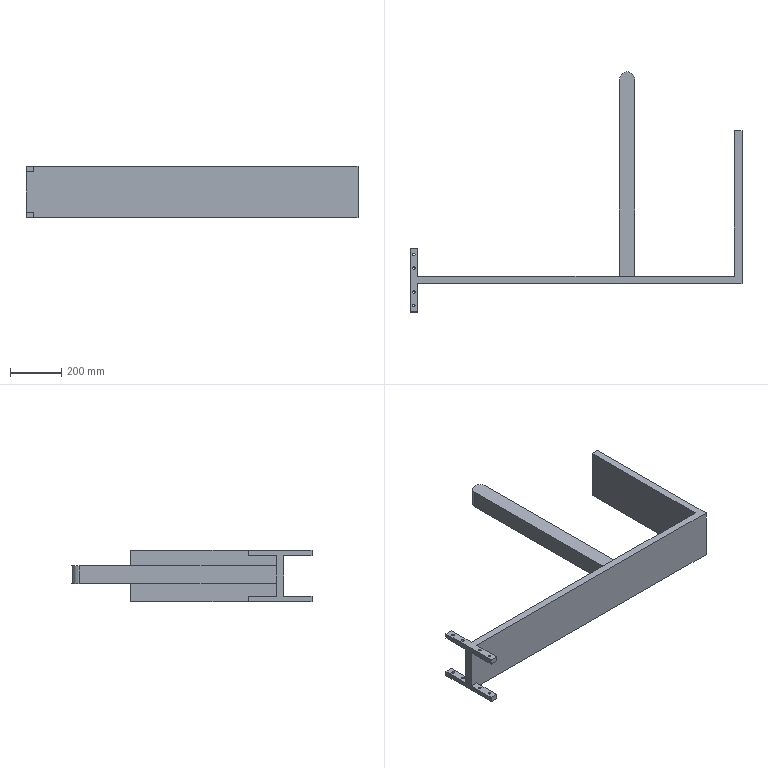Part | SolidWorks | features ICE 3, Extrusion 1 | 1 solid | 41 faces | box 1300 x 940 x 200 mm | volume 14804394 mm3 | plane 24 | cylinder 17 | commonest cylinder face diameters 10 x16 60 x1
STEP:
#1=CARTESIAN_POINT('',(-1438.05,-1320.198,-180.));
#2=VERTEX_POINT('',#1);
#3=CARTESIAN_POINT('',(-1428.05,-1320.198,-180.));
#4=VERTEX_POINT('',#3);
#5=CARTESIAN_POINT('',(-1433.05,-1320.198,-180.));
#6=DIRECTION('',(0.,0.,1.));
#7=DIRECTION('',(0.,-1.,0.));
#8=AXIS2_PLACEMENT_3D('',#5,#6,#7);
#9=CIRCLE('',#8,5.);
#10=EDGE_CURVE('',#2,#4,#9,.T.);
#11=ORIENTED_EDGE('',*,*,#10,.T.);
#12=CARTESIAN_POINT('',(-1428.05,-1320.198,-200.));
#13=VERTEX_POINT('',#12);
#14=CARTESIAN_POINT('',(-1428.05,-1320.198,30.));
#15=DIRECTION('',(0.,0.,-1.));
#16=VECTOR('',#15,1000.);
#17=LINE('',#14,#16);
#18=EDGE_CURVE('',#4,#13,#17,.T.);
#19=ORIENTED_EDGE('',*,*,#18,.T.);
#20=CARTESIAN_POINT('',(-1438.05,-1320.198,-200.));
#21=VERTEX_POINT('',#20);
#22=CARTESIAN_POINT('',(-1433.05,-1320.198,-200.));
#23=DIRECTION('',(0.,0.,-1.));
#24=DIRECTION('',(-1.,0.,0.));
#25=AXIS2_PLACEMENT_3D('',#22,#23,#24);
#26=CIRCLE('',#25,5.);
#27=EDGE_CURVE('',#13,#21,#26,.T.);
#28=ORIENTED_EDGE('',*,*,#27,.T.);
#29=CARTESIAN_POINT('',(-1438.05,-1320.198,30.));
#30=DIRECTION('',(0.,0.,-1.));
#31=VECTOR('',#30,1000.);
#32=LINE('',#29,#31);
#33=EDGE_CURVE('',#2,#21,#32,.T.);
#34=ORIENTED_EDGE('',*,*,#33,.F.);
#35=EDGE_LOOP('',(#11,#19,#28,#34));
#36=FACE_OUTER_BOUND('',#35,.T.);
#37=CARTESIAN_POINT('',(-1433.05,-1320.198,30.));
#38=DIRECTION('',(0.,0.,-1.));
#39=DIRECTION('',(-1.,0.,0.));
#40=AXIS2_PLACEMENT_3D('',#37,#38,#39);
#41=CYLINDRICAL_SURFACE('',#40,5.);
#42=ADVANCED_FACE('',(#36),#41,.F.);
#43=CARTESIAN_POINT('',(-1438.05,-1373.198,-180.));
#44=VERTEX_POINT('',#43);
#45=CARTESIAN_POINT('',(-1428.05,-1373.198,-180.));
#46=VERTEX_POINT('',#45);
#47=CARTESIAN_POINT('',(-1433.05,-1373.198,-180.));
#48=DIRECTION('',(0.,0.,1.));
#49=DIRECTION('',(0.,-1.,0.));
#50=AXIS2_PLACEMENT_3D('',#47,#48,#49);
#51=CIRCLE('',#50,5.);
#52=EDGE_CURVE('',#44,#46,#51,.T.);
#53=ORIENTED_EDGE('',*,*,#52,.T.);
#54=CARTESIAN_POINT('',(-1428.05,-1373.198,-200.));
#55=VERTEX_POINT('',#54);
#56=CARTESIAN_POINT('',(-1428.05,-1373.198,30.));
#57=DIRECTION('',(0.,0.,-1.));
#58=VECTOR('',#57,1000.);
#59=LINE('',#56,#58);
#60=EDGE_CURVE('',#46,#55,#59,.T.);
#61=ORIENTED_EDGE('',*,*,#60,.T.);
#62=CARTESIAN_POINT('',(-1438.05,-1373.198,-200.));
#63=VERTEX_POINT('',#62);
#64=CARTESIAN_POINT('',(-1433.05,-1373.198,-200.));
#65=DIRECTION('',(0.,0.,-1.));
#66=DIRECTION('',(-1.,0.,0.));
#67=AXIS2_PLACEMENT_3D('',#64,#65,#66);
#68=CIRCLE('',#67,5.);
#69=EDGE_CURVE('',#55,#63,#68,.T.);
#70=ORIENTED_EDGE('',*,*,#69,.T.);
#71=CARTESIAN_POINT('',(-1438.05,-1373.198,30.));
#72=DIRECTION('',(0.,0.,-1.));
#73=VECTOR('',#72,1000.);
#74=LINE('',#71,#73);
#75=EDGE_CURVE('',#44,#63,#74,.T.);
#76=ORIENTED_EDGE('',*,*,#75,.F.);
#77=EDGE_LOOP('',(#53,#61,#70,#76));
#78=FACE_OUTER_BOUND('',#77,.T.);
#79=CARTESIAN_POINT('',(-1433.05,-1373.198,30.));
#80=DIRECTION('',(0.,0.,-1.));
#81=DIRECTION('',(-1.,0.,0.));
#82=AXIS2_PLACEMENT_3D('',#79,#80,#81);
#83=CYLINDRICAL_SURFACE('',#82,5.);
#84=ADVANCED_FACE('',(#78),#83,.F.);
#85=CARTESIAN_POINT('',(-1438.05,-1467.198,-180.));
#86=VERTEX_POINT('',#85);
#87=CARTESIAN_POINT('',(-1428.05,-1467.198,-180.));
#88=VERTEX_POINT('',#87);
#89=CARTESIAN_POINT('',(-1433.05,-1467.198,-180.));
#90=DIRECTION('',(0.,0.,1.));
#91=DIRECTION('',(0.,-1.,0.));
#92=AXIS2_PLACEMENT_3D('',#89,#90,#91);
#93=CIRCLE('',#92,5.);
#94=EDGE_CURVE('',#86,#88,#93,.T.);
#95=ORIENTED_EDGE('',*,*,#94,.T.);
#96=CARTESIAN_POINT('',(-1428.05,-1467.198,-200.));
#97=VERTEX_POINT('',#96);
#98=CARTESIAN_POINT('',(-1428.05,-1467.198,30.));
#99=DIRECTION('',(0.,0.,-1.));
#100=VECTOR('',#99,1000.);
#101=LINE('',#98,#100);
#102=EDGE_CURVE('',#88,#97,#101,.T.);
#103=ORIENTED_EDGE('',*,*,#102,.T.);
#104=CARTESIAN_POINT('',(-1438.05,-1467.198,-200.));
#105=VERTEX_POINT('',#104);
#106=CARTESIAN_POINT('',(-1433.05,-1467.198,-200.));
#107=DIRECTION('',(0.,0.,-1.));
#108=DIRECTION('',(1.,0.,0.));
#109=AXIS2_PLACEMENT_3D('',#106,#107,#108);
#110=CIRCLE('',#109,5.);
#111=EDGE_CURVE('',#97,#105,#110,.T.);
#112=ORIENTED_EDGE('',*,*,#111,.T.);
#113=CARTESIAN_POINT('',(-1438.05,-1467.198,30.));
#114=DIRECTION('',(0.,0.,-1.));
#115=VECTOR('',#114,1000.);
#116=LINE('',#113,#115);
#117=EDGE_CURVE('',#86,#105,#116,.T.);
#118=ORIENTED_EDGE('',*,*,#117,.F.);
#119=EDGE_LOOP('',(#95,#103,#112,#118));
#120=FACE_OUTER_BOUND('',#119,.T.);
#121=CARTESIAN_POINT('',(-1433.05,-1467.198,30.));
#122=DIRECTION('',(0.,0.,-1.));
#123=DIRECTION('',(-1.,0.,0.));
#124=AXIS2_PLACEMENT_3D('',#121,#122,#123);
#125=CYLINDRICAL_SURFACE('',#124,5.);
#126=ADVANCED_FACE('',(#120),#125,.F.);
#127=CARTESIAN_POINT('',(-1438.05,-1520.198,-180.));
#128=VERTEX_POINT('',#127);
#129=CARTESIAN_POINT('',(-1428.05,-1520.198,-180.));
#130=VERTEX_POINT('',#129);
#131=CARTESIAN_POINT('',(-1433.05,-1520.198,-180.));
#132=DIRECTION('',(0.,0.,1.));
#133=DIRECTION('',(0.,-1.,0.));
#134=AXIS2_PLACEMENT_3D('',#131,#132,#133);
#135=CIRCLE('',#134,5.);
#136=EDGE_CURVE('',#128,#130,#135,.T.);
#137=ORIENTED_EDGE('',*,*,#136,.T.);
#138=CARTESIAN_POINT('',(-1428.05,-1520.198,-200.));
#139=VERTEX_POINT('',#138);
#140=CARTESIAN_POINT('',(-1428.05,-1520.198,30.));
#141=DIRECTION('',(0.,0.,-1.));
#142=VECTOR('',#141,1000.);
#143=LINE('',#140,#142);
#144=EDGE_CURVE('',#130,#139,#143,.T.);
#145=ORIENTED_EDGE('',*,*,#144,.T.);
#146=CARTESIAN_POINT('',(-1438.05,-1520.198,-200.));
#147=VERTEX_POINT('',#146);
#148=CARTESIAN_POINT('',(-1433.05,-1520.198,-200.));
#149=DIRECTION('',(0.,0.,-1.));
#150=DIRECTION('',(1.,0.,0.));
#151=AXIS2_PLACEMENT_3D('',#148,#149,#150);
#152=CIRCLE('',#151,5.);
#153=EDGE_CURVE('',#139,#147,#152,.T.);
#154=ORIENTED_EDGE('',*,*,#153,.T.);
#155=CARTESIAN_POINT('',(-1438.05,-1520.198,30.));
#156=DIRECTION('',(0.,0.,-1.));
#157=VECTOR('',#156,1000.);
#158=LINE('',#155,#157);
#159=EDGE_CURVE('',#128,#147,#158,.T.);
#160=ORIENTED_EDGE('',*,*,#159,.F.);
#161=EDGE_LOOP('',(#137,#145,#154,#160));
#162=FACE_OUTER_BOUND('',#161,.T.);
#163=CARTESIAN_POINT('',(-1433.05,-1520.198,30.));
#164=DIRECTION('',(0.,0.,-1.));
#165=DIRECTION('',(-1.,0.,0.));
#166=AXIS2_PLACEMENT_3D('',#163,#164,#165);
#167=CYLINDRICAL_SURFACE('',#166,5.);
#168=ADVANCED_FACE('',(#162),#167,.F.);
#169=CARTESIAN_POINT('',(-1428.05,-1320.198,0.));
#170=VERTEX_POINT('',#169);
#171=CARTESIAN_POINT('',(-1438.05,-1320.198,0.));
#172=VERTEX_POINT('',#171);
#173=CARTESIAN_POINT('',(-1433.05,-1320.198,0.));
#174=DIRECTION('',(0.,0.,-1.));
#175=DIRECTION('',(-1.,0.,0.));
#176=AXIS2_PLACEMENT_3D('',#173,#174,#175);
#177=CIRCLE('',#176,5.);
#178=EDGE_CURVE('',#170,#172,#177,.T.);
#179=ORIENTED_EDGE('',*,*,#178,.F.);
#180=CARTESIAN_POINT('',(-1428.05,-1320.198,-20.));
#181=VERTEX_POINT('',#180);
#182=CARTESIAN_POINT('',(-1428.05,-1320.198,30.));
#183=DIRECTION('',(0.,0.,-1.));
#184=VECTOR('',#183,1000.);
#185=LINE('',#182,#184);
#186=EDGE_CURVE('',#170,#181,#185,.T.);
#187=ORIENTED_EDGE('',*,*,#186,.T.);
#188=CARTESIAN_POINT('',(-1438.05,-1320.198,-20.));
#189=VERTEX_POINT('',#188);
#190=CARTESIAN_POINT('',(-1433.05,-1320.198,-20.));
#191=DIRECTION('',(0.,0.,-1.));
#192=DIRECTION('',(0.,1.,0.));
#193=AXIS2_PLACEMENT_3D('',#190,#191,#192);
#194=CIRCLE('',#193,5.);
#195=EDGE_CURVE('',#181,#189,#194,.T.);
#196=ORIENTED_EDGE('',*,*,#195,.T.);
#197=CARTESIAN_POINT('',(-1438.05,-1320.198,30.));
#198=DIRECTION('',(0.,0.,-1.));
#199=VECTOR('',#198,1000.);
#200=LINE('',#197,#199);
#201=EDGE_CURVE('',#172,#189,#200,.T.);
#202=ORIENTED_EDGE('',*,*,#201,.F.);
#203=EDGE_LOOP('',(#179,#187,#196,#202));
#204=FACE_OUTER_BOUND('',#203,.T.);
#205=CARTESIAN_POINT('',(-1433.05,-1320.198,30.));
#206=DIRECTION('',(0.,0.,-1.));
#207=DIRECTION('',(-1.,0.,0.));
#208=AXIS2_PLACEMENT_3D('',#205,#206,#207);
#209=CYLINDRICAL_SURFACE('',#208,5.);
#210=ADVANCED_FACE('',(#204),#209,.F.);
#211=CARTESIAN_POINT('',(-1428.05,-1373.198,0.));
#212=VERTEX_POINT('',#211);
#213=CARTESIAN_POINT('',(-1438.05,-1373.198,0.));
#214=VERTEX_POINT('',#213);
#215=CARTESIAN_POINT('',(-1433.05,-1373.198,0.));
#216=DIRECTION('',(0.,0.,-1.));
#217=DIRECTION('',(-1.,0.,0.));
#218=AXIS2_PLACEMENT_3D('',#215,#216,#217);
#219=CIRCLE('',#218,5.);
#220=EDGE_CURVE('',#212,#214,#219,.T.);
#221=ORIENTED_EDGE('',*,*,#220,.F.);
#222=CARTESIAN_POINT('',(-1428.05,-1373.198,-20.));
#223=VERTEX_POINT('',#222);
#224=CARTESIAN_POINT('',(-1428.05,-1373.198,30.));
#225=DIRECTION('',(0.,0.,-1.));
#226=VECTOR('',#225,1000.);
#227=LINE('',#224,#226);
#228=EDGE_CURVE('',#212,#223,#227,.T.);
#229=ORIENTED_EDGE('',*,*,#228,.T.);
#230=CARTESIAN_POINT('',(-1438.05,-1373.198,-20.));
#231=VERTEX_POINT('',#230);
#232=CARTESIAN_POINT('',(-1433.05,-1373.198,-20.));
#233=DIRECTION('',(0.,0.,-1.));
#234=DIRECTION('',(0.,1.,0.));
#235=AXIS2_PLACEMENT_3D('',#232,#233,#234);
#236=CIRCLE('',#235,5.);
#237=EDGE_CURVE('',#223,#231,#236,.T.);
#238=ORIENTED_EDGE('',*,*,#237,.T.);
#239=CARTESIAN_POINT('',(-1438.05,-1373.198,30.));
#240=DIRECTION('',(0.,0.,-1.));
#241=VECTOR('',#240,1000.);
#242=LINE('',#239,#241);
#243=EDGE_CURVE('',#214,#231,#242,.T.);
#244=ORIENTED_EDGE('',*,*,#243,.F.);
#245=EDGE_LOOP('',(#221,#229,#238,#244));
#246=FACE_OUTER_BOUND('',#245,.T.);
#247=CARTESIAN_POINT('',(-1433.05,-1373.198,30.));
#248=DIRECTION('',(0.,0.,-1.));
#249=DIRECTION('',(-1.,0.,0.));
#250=AXIS2_PLACEMENT_3D('',#247,#248,#249);
#251=CYLINDRICAL_SURFACE('',#250,5.);
#252=ADVANCED_FACE('',(#246),#251,.F.);
#253=CARTESIAN_POINT('',(-1428.05,-1467.198,0.));
#254=VERTEX_POINT('',#253);
#255=CARTESIAN_POINT('',(-1438.05,-1467.198,0.));
#256=VERTEX_POINT('',#255);
#257=CARTESIAN_POINT('',(-1433.05,-1467.198,0.));
#258=DIRECTION('',(0.,0.,-1.));
#259=DIRECTION('',(-1.,0.,0.));
#260=AXIS2_PLACEMENT_3D('',#257,#258,#259);
#261=CIRCLE('',#260,5.);
#262=EDGE_CURVE('',#254,#256,#261,.T.);
#263=ORIENTED_EDGE('',*,*,#262,.F.);
#264=CARTESIAN_POINT('',(-1428.05,-1467.198,-20.));
#265=VERTEX_POINT('',#264);
#266=CARTESIAN_POINT('',(-1428.05,-1467.198,30.));
#267=DIRECTION('',(0.,0.,-1.));
#268=VECTOR('',#267,1000.);
#269=LINE('',#266,#268);
#270=EDGE_CURVE('',#254,#265,#269,.T.);
#271=ORIENTED_EDGE('',*,*,#270,.T.);
#272=CARTESIAN_POINT('',(-1438.05,-1467.198,-20.));
#273=VERTEX_POINT('',#272);
#274=CARTESIAN_POINT('',(-1433.05,-1467.198,-20.));
#275=DIRECTION('',(0.,0.,-1.));
#276=DIRECTION('',(0.,1.,0.));
#277=AXIS2_PLACEMENT_3D('',#274,#275,#276);
#278=CIRCLE('',#277,5.);
#279=EDGE_CURVE('',#265,#273,#278,.T.);
#280=ORIENTED_EDGE('',*,*,#279,.T.);
#281=CARTESIAN_POINT('',(-1438.05,-1467.198,30.));
#282=DIRECTION('',(0.,0.,-1.));
#283=VECTOR('',#282,1000.);
#284=LINE('',#281,#283);
#285=EDGE_CURVE('',#256,#273,#284,.T.);
#286=ORIENTED_EDGE('',*,*,#285,.F.);
#287=EDGE_LOOP('',(#263,#271,#280,#286));
#288=FACE_OUTER_BOUND('',#287,.T.);
#289=CARTESIAN_POINT('',(-1433.05,-1467.198,30.));
#290=DIRECTION('',(0.,0.,-1.));
#291=DIRECTION('',(-1.,0.,0.));
#292=AXIS2_PLACEMENT_3D('',#289,#290,#291);
#293=CYLINDRICAL_SURFACE('',#292,5.);
#294=ADVANCED_FACE('',(#288),#293,.F.);
#295=CARTESIAN_POINT('',(-1428.05,-1520.198,0.));
#296=VERTEX_POINT('',#295);
#297=CARTESIAN_POINT('',(-1438.05,-1520.198,0.));
#298=VERTEX_POINT('',#297);
#299=CARTESIAN_POINT('',(-1433.05,-1520.198,0.));
#300=DIRECTION('',(0.,0.,-1.));
#301=DIRECTION('',(-1.,0.,0.));
#302=AXIS2_PLACEMENT_3D('',#299,#300,#301);
#303=CIRCLE('',#302,5.);
#304=EDGE_CURVE('',#296,#298,#303,.T.);
#305=ORIENTED_EDGE('',*,*,#304,.F.);
#306=CARTESIAN_POINT('',(-1428.05,-1520.198,-20.));
#307=VERTEX_POINT('',#306);
#308=CARTESIAN_POINT('',(-1428.05,-1520.198,30.));
#309=DIRECTION('',(0.,0.,-1.));
#310=VECTOR('',#309,1000.);
#311=LINE('',#308,#310);
#312=EDGE_CURVE('',#296,#307,#311,.T.);
#313=ORIENTED_EDGE('',*,*,#312,.T.);
#314=CARTESIAN_POINT('',(-1438.05,-1520.198,-20.));
#315=VERTEX_POINT('',#314);
#316=CARTESIAN_POINT('',(-1433.05,-1520.198,-20.));
#317=DIRECTION('',(0.,0.,-1.));
#318=DIRECTION('',(0.,1.,0.));
#319=AXIS2_PLACEMENT_3D('',#316,#317,#318);
#320=CIRCLE('',#319,5.);
#321=EDGE_CURVE('',#307,#315,#320,.T.);
#322=ORIENTED_EDGE('',*,*,#321,.T.);
#323=CARTESIAN_POINT('',(-1438.05,-1520.198,30.));
#324=DIRECTION('',(0.,0.,-1.));
#325=VECTOR('',#324,1000.);
#326=LINE('',#323,#325);
#327=EDGE_CURVE('',#298,#315,#326,.T.);
#328=ORIENTED_EDGE('',*,*,#327,.F.);
#329=EDGE_LOOP('',(#305,#313,#322,#328));
#330=FACE_OUTER_BOUND('',#329,.T.);
#331=CARTESIAN_POINT('',(-1433.05,-1520.198,30.));
#332=DIRECTION('',(0.,0.,-1.));
#333=DIRECTION('',(-1.,0.,0.));
#334=AXIS2_PLACEMENT_3D('',#331,#332,#333);
#335=CYLINDRICAL_SURFACE('',#334,5.);
#336=ADVANCED_FACE('',(#330),#335,.F.);
#337=CARTESIAN_POINT('',(-1418.05,-1405.198,-20.));
#338=VERTEX_POINT('',#337);
#339=CARTESIAN_POINT('',(-1448.05,-1405.198,-20.));
#340=VERTEX_POINT('',#339);
#341=CARTESIAN_POINT('',(-178.05,-1405.198,-20.));
#342=DIRECTION('',(-1.,0.,0.));
#343=VECTOR('',#342,1000.);
#344=LINE('',#341,#343);
#345=EDGE_CURVE('',#338,#340,#344,.T.);
#346=ORIENTED_EDGE('',*,*,#345,.F.);
#347=CARTESIAN_POINT('',(-1418.05,-1405.198,0.));
#348=VERTEX_POINT('',#347);
#349=CARTESIAN_POINT('',(-1418.05,-1405.198,-200.));
#350=DIRECTION('',(0.,0.,-1.));
#351=VECTOR('',#350,1000.);
#352=LINE('',#349,#351);
#353=EDGE_CURVE('',#348,#338,#352,.T.);
#354=ORIENTED_EDGE('',*,*,#353,.F.);
#355=CARTESIAN_POINT('',(-178.05,-1405.198,0.));
#356=VERTEX_POINT('',#355);
#357=CARTESIAN_POINT('',(-178.05,-1405.198,0.));
#358=DIRECTION('',(-1.,0.,0.));
#359=VECTOR('',#358,1000.);
#360=LINE('',#357,#359);
#361=EDGE_CURVE('',#356,#348,#360,.T.);
#362=ORIENTED_EDGE('',*,*,#361,.F.);
#363=CARTESIAN_POINT('',(-178.05,-1405.198,-200.));
#364=VERTEX_POINT('',#363);
#365=CARTESIAN_POINT('',(-178.05,-1405.198,-200.));
#366=DIRECTION('',(0.,0.,1.));
#367=VECTOR('',#366,1000.);
#368=LINE('',#365,#367);
#369=EDGE_CURVE('',#364,#356,#368,.T.);
#370=ORIENTED_EDGE('',*,*,#369,.F.);
#371=CARTESIAN_POINT('',(-1418.05,-1405.198,-200.));
#372=VERTEX_POINT('',#371);
#373=CARTESIAN_POINT('',(-178.05,-1405.198,-200.));
#374=DIRECTION('',(-1.,0.,0.));
#375=VECTOR('',#374,1000.);
#376=LINE('',#373,#375);
#377=EDGE_CURVE('',#364,#372,#376,.T.);
#378=ORIENTED_EDGE('',*,*,#377,.T.);
#379=CARTESIAN_POINT('',(-1418.05,-1405.198,-180.));
#380=VERTEX_POINT('',#379);
#381=CARTESIAN_POINT('',(-1418.05,-1405.198,-200.));
#382=DIRECTION('',(0.,0.,-1.));
#383=VECTOR('',#382,1000.);
#384=LINE('',#381,#383);
#385=EDGE_CURVE('',#380,#372,#384,.T.);
#386=ORIENTED_EDGE('',*,*,#385,.F.);
#387=CARTESIAN_POINT('',(-1448.05,-1405.198,-180.));
#388=VERTEX_POINT('',#387);
#389=CARTESIAN_POINT('',(-178.05,-1405.198,-180.));
#390=DIRECTION('',(1.,0.,0.));
#391=VECTOR('',#390,1000.);
#392=LINE('',#389,#391);
#393=EDGE_CURVE('',#388,#380,#392,.T.);
#394=ORIENTED_EDGE('',*,*,#393,.F.);
#395=CARTESIAN_POINT('',(-1448.05,-1405.198,-200.));
#396=DIRECTION('',(0.,0.,1.));
#397=VECTOR('',#396,1000.);
#398=LINE('',#395,#397);
#399=EDGE_CURVE('',#388,#340,#398,.T.);
#400=ORIENTED_EDGE('',*,*,#399,.T.);
#401=EDGE_LOOP('',(#346,#354,#362,#370,#378,#386,#394,#400));
#402=FACE_OUTER_BOUND('',#401,.T.);
#403=CARTESIAN_POINT('',(-628.05,-1405.198,-130.));
#404=VERTEX_POINT('',#403);
#405=CARTESIAN_POINT('',(-628.05,-1405.198,-60.));
#406=VERTEX_POINT('',#405);
#407=CARTESIAN_POINT('',(-628.05,-1405.198,-130.));
#408=DIRECTION('',(0.,0.,1.));
#409=VECTOR('',#408,1000.);
#410=LINE('',#407,#409);
#411=EDGE_CURVE('',#404,#406,#410,.T.);
#412=ORIENTED_EDGE('',*,*,#411,.F.);
#413=CARTESIAN_POINT('',(-568.05,-1405.198,-130.));
#414=VERTEX_POINT('',#413);
#415=CARTESIAN_POINT('',(-568.05,-1405.198,-130.));
#416=DIRECTION('',(1.,0.,0.));
#417=VECTOR('',#416,1000.);
#418=LINE('',#415,#417);
#419=EDGE_CURVE('',#404,#414,#418,.T.);
#420=ORIENTED_EDGE('',*,*,#419,.T.);
#421=CARTESIAN_POINT('',(-568.05,-1405.198,-60.));
#422=VERTEX_POINT('',#421);
#423=CARTESIAN_POINT('',(-568.05,-1405.198,-130.));
#424=DIRECTION('',(0.,0.,1.));
#425=VECTOR('',#424,1000.);
#426=LINE('',#423,#425);
#427=EDGE_CURVE('',#414,#422,#426,.T.);
#428=ORIENTED_EDGE('',*,*,#427,.T.);
#429=CARTESIAN_POINT('',(-568.05,-1405.198,-60.));
#430=DIRECTION('',(1.,0.,0.));
#431=VECTOR('',#430,1000.);
#432=LINE('',#429,#431);
#433=EDGE_CURVE('',#406,#422,#432,.T.);
#434=ORIENTED_EDGE('',*,*,#433,.F.);
#435=EDGE_LOOP('',(#412,#420,#428,#434));
#436=FACE_BOUND('',#435,.T.);
#437=CARTESIAN_POINT('',(-178.05,-1405.198,-200.));
#438=DIRECTION('',(0.,1.,0.));
#439=DIRECTION('',(0.,0.,1.));
#440=AXIS2_PLACEMENT_3D('',#437,#438,#439);
#441=PLANE('',#440);
#442=ADVANCED_FACE('',(#402,#436),#441,.T.);
#443=CARTESIAN_POINT('',(-148.05,-1435.198,0.));
#444=VERTEX_POINT('',#443);
#445=CARTESIAN_POINT('',(-148.05,-835.198,0.));
#446=VERTEX_POINT('',#445);
#447=CARTESIAN_POINT('',(-148.05,-835.198,0.));
#448=DIRECTION('',(0.,1.,0.));
#449=VECTOR('',#448,1000.);
#450=LINE('',#447,#449);
#451=EDGE_CURVE('',#444,#446,#450,.T.);
#452=ORIENTED_EDGE('',*,*,#451,.F.);
#453=CARTESIAN_POINT('',(-148.05,-1435.198,-200.));
#454=VERTEX_POINT('',#453);
#455=CARTESIAN_POINT('',(-148.05,-1435.198,-200.));
#456=DIRECTION('',(0.,0.,1.));
#457=VECTOR('',#456,1000.);
#458=LINE('',#455,#457);
#459=EDGE_CURVE('',#454,#444,#458,.T.);
#460=ORIENTED_EDGE('',*,*,#459,.F.);
#461=CARTESIAN_POINT('',(-148.05,-835.198,-200.));
#462=VERTEX_POINT('',#461);
#463=CARTESIAN_POINT('',(-148.05,-835.198,-200.));
#464=DIRECTION('',(0.,1.,0.));
#465=VECTOR('',#464,1000.);
#466=LINE('',#463,#465);
#467=EDGE_CURVE('',#454,#462,#466,.T.);
#468=ORIENTED_EDGE('',*,*,#467,.T.);
#469=CARTESIAN_POINT('',(-148.05,-835.198,-200.));
#470=DIRECTION('',(0.,0.,1.));
#471=VECTOR('',#470,1000.);
#472=LINE('',#469,#471);
#473=EDGE_CURVE('',#462,#446,#472,.T.);
#474=ORIENTED_EDGE('',*,*,#473,.T.);
#475=EDGE_LOOP('',(#452,#460,#468,#474));
#476=FACE_OUTER_BOUND('',#475,.T.);
#477=CARTESIAN_POINT('',(-148.05,-835.198,-200.));
#478=DIRECTION('',(1.,0.,0.));
#479=DIRECTION('',(0.,1.,0.));
#480=AXIS2_PLACEMENT_3D('',#477,#478,#479);
#481=PLANE('',#480);
#482=ADVANCED_FACE('',(#476),#481,.T.);
#483=CARTESIAN_POINT('',(-1448.05,-1435.198,-20.));
#484=VERTEX_POINT('',#483);
#485=CARTESIAN_POINT('',(-1418.05,-1435.198,-20.));
#486=VERTEX_POINT('',#485);
#487=CARTESIAN_POINT('',(-148.05,-1435.198,-20.));
#488=DIRECTION('',(1.,0.,0.));
#489=VECTOR('',#488,1000.);
#490=LINE('',#487,#489);
#491=EDGE_CURVE('',#484,#486,#490,.T.);
#492=ORIENTED_EDGE('',*,*,#491,.F.);
#493=CARTESIAN_POINT('',(-1448.05,-1435.198,-180.));
#494=VERTEX_POINT('',#493);
#495=CARTESIAN_POINT('',(-1448.05,-1435.198,-200.));
#496=DIRECTION('',(0.,0.,1.));
#497=VECTOR('',#496,1000.);
#498=LINE('',#495,#497);
#499=EDGE_CURVE('',#494,#484,#498,.T.);
#500=ORIENTED_EDGE('',*,*,#499,.F.);
#501=CARTESIAN_POINT('',(-1418.05,-1435.198,-180.));
#502=VERTEX_POINT('',#501);
#503=CARTESIAN_POINT('',(-148.05,-1435.198,-180.));
#504=DIRECTION('',(-1.,0.,0.));
#505=VECTOR('',#504,1000.);
#506=LINE('',#503,#505);
#507=EDGE_CURVE('',#502,#494,#506,.T.);
#508=ORIENTED_EDGE('',*,*,#507,.F.);
#509=CARTESIAN_POINT('',(-1418.05,-1435.198,-200.));
#510=VERTEX_POINT('',#509);
#511=CARTESIAN_POINT('',(-1418.05,-1435.198,-200.));
#512=DIRECTION('',(0.,0.,1.));
#513=VECTOR('',#512,1000.);
#514=LINE('',#511,#513);
#515=EDGE_CURVE('',#510,#502,#514,.T.);
#516=ORIENTED_EDGE('',*,*,#515,.F.);
#517=CARTESIAN_POINT('',(-148.05,-1435.198,-200.));
#518=DIRECTION('',(1.,0.,0.));
#519=VECTOR('',#518,1000.);
#520=LINE('',#517,#519);
#521=EDGE_CURVE('',#510,#454,#520,.T.);
#522=ORIENTED_EDGE('',*,*,#521,.T.);
#523=ORIENTED_EDGE('',*,*,#459,.T.);
#524=CARTESIAN_POINT('',(-1418.05,-1435.198,0.));
#525=VERTEX_POINT('',#524);
#526=CARTESIAN_POINT('',(-148.05,-1435.198,0.));
#527=DIRECTION('',(1.,0.,0.));
#528=VECTOR('',#527,1000.);
#529=LINE('',#526,#528);
#530=EDGE_CURVE('',#525,#444,#529,.T.);
#531=ORIENTED_EDGE('',*,*,#530,.F.);
#532=CARTESIAN_POINT('',(-1418.05,-1435.198,-200.));
#533=DIRECTION('',(0.,0.,1.));
#534=VECTOR('',#533,1000.);
#535=LINE('',#532,#534);
#536=EDGE_CURVE('',#486,#525,#535,.T.);
#537=ORIENTED_EDGE('',*,*,#536,.F.);
#538=EDGE_LOOP('',(#492,#500,#508,#516,#522,#523,#531,#537));
#539=FACE_OUTER_BOUND('',#538,.T.);
#540=CARTESIAN_POINT('',(-148.05,-1435.198,-200.));
#541=DIRECTION('',(0.,-1.,0.));
#542=DIRECTION('',(0.,0.,-1.));
#543=AXIS2_PLACEMENT_3D('',#540,#541,#542);
#544=PLANE('',#543);
#545=ADVANCED_FACE('',(#539),#544,.T.);
#546=ORIENTED_EDGE('',*,*,#499,.T.);
#547=CARTESIAN_POINT('',(-1448.05,-1545.198,-20.));
#548=VERTEX_POINT('',#547);
#549=CARTESIAN_POINT('',(-1448.05,-1295.198,-20.));
#550=DIRECTION('',(0.,-1.,0.));
#551=VECTOR('',#550,1000.);
#552=LINE('',#549,#551);
#553=EDGE_CURVE('',#484,#548,#552,.T.);
#554=ORIENTED_EDGE('',*,*,#553,.T.);
#555=CARTESIAN_POINT('',(-1448.05,-1545.198,0.));
#556=VERTEX_POINT('',#555);
#557=CARTESIAN_POINT('',(-1448.05,-1545.198,-20.));
#558=DIRECTION('',(0.,0.,1.));
#559=VECTOR('',#558,1000.);
#560=LINE('',#557,#559);
#561=EDGE_CURVE('',#548,#556,#560,.T.);
#562=ORIENTED_EDGE('',*,*,#561,.T.);
#563=CARTESIAN_POINT('',(-1448.05,-1295.198,0.));
#564=VERTEX_POINT('',#563);
#565=CARTESIAN_POINT('',(-1448.05,-1435.198,0.));
#566=DIRECTION('',(0.,-1.,0.));
#567=VECTOR('',#566,1000.);
#568=LINE('',#565,#567);
#569=EDGE_CURVE('',#564,#556,#568,.T.);
#570=ORIENTED_EDGE('',*,*,#569,.F.);
#571=CARTESIAN_POINT('',(-1448.05,-1295.198,-20.));
#572=VERTEX_POINT('',#571);
#573=CARTESIAN_POINT('',(-1448.05,-1295.198,-20.));
#574=DIRECTION('',(0.,0.,-1.));
#575=VECTOR('',#574,1000.);
#576=LINE('',#573,#575);
#577=EDGE_CURVE('',#564,#572,#576,.T.);
#578=ORIENTED_EDGE('',*,*,#577,.T.);
#579=CARTESIAN_POINT('',(-1448.05,-1295.198,-20.));
#580=DIRECTION('',(0.,-1.,0.));
#581=VECTOR('',#580,1000.);
#582=LINE('',#579,#581);
#583=EDGE_CURVE('',#572,#340,#582,.T.);
#584=ORIENTED_EDGE('',*,*,#583,.T.);
#585=ORIENTED_EDGE('',*,*,#399,.F.);
#586=CARTESIAN_POINT('',(-1448.05,-1295.198,-180.));
#587=VERTEX_POINT('',#586);
#588=CARTESIAN_POINT('',(-1448.05,-1295.198,-180.));
#589=DIRECTION('',(0.,1.,0.));
#590=VECTOR('',#589,1000.);
#591=LINE('',#588,#590);
#592=EDGE_CURVE('',#388,#587,#591,.T.);
#593=ORIENTED_EDGE('',*,*,#592,.T.);
#594=CARTESIAN_POINT('',(-1448.05,-1295.198,-200.));
#595=VERTEX_POINT('',#594);
#596=CARTESIAN_POINT('',(-1448.05,-1295.198,-180.));
#597=DIRECTION('',(0.,0.,-1.));
#598=VECTOR('',#597,1000.);
#599=LINE('',#596,#598);
#600=EDGE_CURVE('',#587,#595,#599,.T.);
#601=ORIENTED_EDGE('',*,*,#600,.T.);
#602=CARTESIAN_POINT('',(-1448.05,-1545.198,-200.));
#603=VERTEX_POINT('',#602);
#604=CARTESIAN_POINT('',(-1448.05,-1435.198,-200.));
#605=DIRECTION('',(0.,-1.,0.));
#606=VECTOR('',#605,1000.);
#607=LINE('',#604,#606);
#608=EDGE_CURVE('',#595,#603,#607,.T.);
#609=ORIENTED_EDGE('',*,*,#608,.T.);
#610=CARTESIAN_POINT('',(-1448.05,-1545.198,-180.));
#611=VERTEX_POINT('',#610);
#612=CARTESIAN_POINT('',(-1448.05,-1545.198,-180.));
#613=DIRECTION('',(0.,0.,1.));
#614=VECTOR('',#613,1000.);
#615=LINE('',#612,#614);
#616=EDGE_CURVE('',#603,#611,#615,.T.);
#617=ORIENTED_EDGE('',*,*,#616,.T.);
#618=CARTESIAN_POINT('',(-1448.05,-1295.198,-180.));
#619=DIRECTION('',(0.,1.,0.));
#620=VECTOR('',#619,1000.);
#621=LINE('',#618,#620);
#622=EDGE_CURVE('',#611,#494,#621,.T.);
#623=ORIENTED_EDGE('',*,*,#622,.T.);
#624=EDGE_LOOP('',(#546,#554,#562,#570,#578,#584,#585,#593,#601,#609,#617,#623));
#625=FACE_OUTER_BOUND('',#624,.T.);
#626=CARTESIAN_POINT('',(-1448.05,-1435.198,-200.));
#627=DIRECTION('',(-1.,0.,0.));
#628=DIRECTION('',(0.,-1.,0.));
#629=AXIS2_PLACEMENT_3D('',#626,#627,#628);
#630=PLANE('',#629);
#631=ADVANCED_FACE('',(#625),#630,.T.);
#632=CARTESIAN_POINT('',(-178.05,-835.198,0.));
#633=VERTEX_POINT('',#632);
#634=CARTESIAN_POINT('',(-178.05,-835.198,0.));
#635=DIRECTION('',(0.,-1.,0.));
#636=VECTOR('',#635,1000.);
#637=LINE('',#634,#636);
#638=EDGE_CURVE('',#633,#356,#637,.T.);
#639=ORIENTED_EDGE('',*,*,#638,.F.);
#640=CARTESIAN_POINT('',(-178.05,-835.198,-200.));
#641=VERTEX_POINT('',#640);
#642=CARTESIAN_POINT('',(-178.05,-835.198,-200.));
#643=DIRECTION('',(0.,0.,1.));
#644=VECTOR('',#643,1000.);
#645=LINE('',#642,#644);
#646=EDGE_CURVE('',#641,#633,#645,.T.);
#647=ORIENTED_EDGE('',*,*,#646,.F.);
#648=CARTESIAN_POINT('',(-178.05,-835.198,-200.));
#649=DIRECTION('',(0.,-1.,0.));
#650=VECTOR('',#649,1000.);
#651=LINE('',#648,#650);
#652=EDGE_CURVE('',#641,#364,#651,.T.);
#653=ORIENTED_EDGE('',*,*,#652,.T.);
#654=ORIENTED_EDGE('',*,*,#369,.T.);
#655=EDGE_LOOP('',(#639,#647,#653,#654));
#656=FACE_OUTER_BOUND('',#655,.T.);
#657=CARTESIAN_POINT('',(-178.05,-835.198,-200.));
#658=DIRECTION('',(-1.,0.,0.));
#659=DIRECTION('',(0.,-1.,0.));
#660=AXIS2_PLACEMENT_3D('',#657,#658,#659);
#661=PLANE('',#660);
#662=ADVANCED_FACE('',(#656),#661,.T.);
#663=CARTESIAN_POINT('',(-148.05,-835.198,0.));
#664=DIRECTION('',(-1.,0.,0.));
#665=VECTOR('',#664,1000.);
#666=LINE('',#663,#665);
#667=EDGE_CURVE('',#446,#633,#666,.T.);
#668=ORIENTED_EDGE('',*,*,#667,.F.);
#669=ORIENTED_EDGE('',*,*,#473,.F.);
#670=CARTESIAN_POINT('',(-148.05,-835.198,-200.));
#671=DIRECTION('',(-1.,0.,0.));
#672=VECTOR('',#671,1000.);
#673=LINE('',#670,#672);
#674=EDGE_CURVE('',#462,#641,#673,.T.);
#675=ORIENTED_EDGE('',*,*,#674,.T.);
#676=ORIENTED_EDGE('',*,*,#646,.T.);
#677=EDGE_LOOP('',(#668,#669,#675,#676));
#678=FACE_OUTER_BOUND('',#677,.T.);
#679=CARTESIAN_POINT('',(-148.05,-835.198,-200.));
#680=DIRECTION('',(0.,1.,0.));
#681=DIRECTION('',(0.,0.,1.));
#682=AXIS2_PLACEMENT_3D('',#679,#680,#681);
#683=PLANE('',#682);
#684=ADVANCED_FACE('',(#678),#683,.T.);
#685=CARTESIAN_POINT('',(-1433.05,-1320.198,-200.));
#686=DIRECTION('',(0.,0.,-1.));
#687=DIRECTION('',(-1.,0.,0.));
#688=AXIS2_PLACEMENT_3D('',#685,#686,#687);
#689=CIRCLE('',#688,5.);
#690=EDGE_CURVE('',#21,#13,#689,.T.);
#691=ORIENTED_EDGE('',*,*,#690,.F.);
#692=ORIENTED_EDGE('',*,*,#27,.F.);
#693=EDGE_LOOP('',(#691,#692));
#694=FACE_BOUND('',#693,.T.);
#695=CARTESIAN_POINT('',(-1433.05,-1467.198,-200.));
#696=DIRECTION('',(0.,0.,-1.));
#697=DIRECTION('',(1.,0.,0.));
#698=AXIS2_PLACEMENT_3D('',#695,#696,#697);
#699=CIRCLE('',#698,5.);
#700=EDGE_CURVE('',#105,#97,#699,.T.);
#701=ORIENTED_EDGE('',*,*,#700,.F.);
#702=ORIENTED_EDGE('',*,*,#111,.F.);
#703=EDGE_LOOP('',(#701,#702));
#704=FACE_BOUND('',#703,.T.);
#705=CARTESIAN_POINT('',(-1433.05,-1520.198,-200.));
#706=DIRECTION('',(0.,0.,-1.));
#707=DIRECTION('',(1.,0.,0.));
#708=AXIS2_PLACEMENT_3D('',#705,#706,#707);
#709=CIRCLE('',#708,5.);
#710=EDGE_CURVE('',#147,#139,#709,.T.);
#711=ORIENTED_EDGE('',*,*,#710,.F.);
#712=ORIENTED_EDGE('',*,*,#153,.F.);
#713=EDGE_LOOP('',(#711,#712));
#714=FACE_BOUND('',#713,.T.);
#715=CARTESIAN_POINT('',(-1433.05,-1373.198,-200.));
#716=DIRECTION('',(0.,0.,-1.));
#717=DIRECTION('',(-1.,0.,0.));
#718=AXIS2_PLACEMENT_3D('',#715,#716,#717);
#719=CIRCLE('',#718,5.);
#720=EDGE_CURVE('',#63,#55,#719,.T.);
#721=ORIENTED_EDGE('',*,*,#720,.F.);
#722=ORIENTED_EDGE('',*,*,#69,.F.);
#723=EDGE_LOOP('',(#721,#722));
#724=FACE_BOUND('',#723,.T.);
#725=ORIENTED_EDGE('',*,*,#521,.F.);
#726=CARTESIAN_POINT('',(-1418.05,-1545.198,-200.));
#727=VERTEX_POINT('',#726);
#728=CARTESIAN_POINT('',(-1418.05,-1295.198,-200.));
#729=DIRECTION('',(0.,-1.,0.));
#730=VECTOR('',#729,1000.);
#731=LINE('',#728,#730);
#732=EDGE_CURVE('',#510,#727,#731,.T.);
#733=ORIENTED_EDGE('',*,*,#732,.T.);
#734=CARTESIAN_POINT('',(-1418.05,-1545.198,-200.));
#735=DIRECTION('',(-1.,0.,0.));
#736=VECTOR('',#735,1000.);
#737=LINE('',#734,#736);
#738=EDGE_CURVE('',#727,#603,#737,.T.);
#739=ORIENTED_EDGE('',*,*,#738,.T.);
#740=ORIENTED_EDGE('',*,*,#608,.F.);
#741=CARTESIAN_POINT('',(-1418.05,-1295.198,-200.));
#742=VERTEX_POINT('',#741);
#743=CARTESIAN_POINT('',(-1418.05,-1295.198,-200.));
#744=DIRECTION('',(-1.,0.,0.));
#745=VECTOR('',#744,1000.);
#746=LINE('',#743,#745);
#747=EDGE_CURVE('',#742,#595,#746,.T.);
#748=ORIENTED_EDGE('',*,*,#747,.F.);
#749=CARTESIAN_POINT('',(-1418.05,-1295.198,-200.));
#750=DIRECTION('',(0.,-1.,0.));
#751=VECTOR('',#750,1000.);
#752=LINE('',#749,#751);
#753=EDGE_CURVE('',#742,#372,#752,.T.);
#754=ORIENTED_EDGE('',*,*,#753,.T.);
#755=ORIENTED_EDGE('',*,*,#377,.F.);
#756=ORIENTED_EDGE('',*,*,#652,.F.);
#757=ORIENTED_EDGE('',*,*,#674,.F.);
#758=ORIENTED_EDGE('',*,*,#467,.F.);
#759=EDGE_LOOP('',(#725,#733,#739,#740,#748,#754,#755,#756,#757,#758));
#760=FACE_OUTER_BOUND('',#759,.T.);
#761=CARTESIAN_POINT('',(0.,0.,-200.));
#762=DIRECTION('',(0.,0.,-1.));
#763=DIRECTION('',(-1.,0.,0.));
#764=AXIS2_PLACEMENT_3D('',#761,#762,#763);
#765=PLANE('',#764);
#766=ADVANCED_FACE('',(#694,#704,#714,#724,#760),#765,.T.);
#767=CARTESIAN_POINT('',(-1433.05,-1320.198,0.));
#768=DIRECTION('',(0.,0.,-1.));
#769=DIRECTION('',(-1.,0.,0.));
#770=AXIS2_PLACEMENT_3D('',#767,#768,#769);
#771=CIRCLE('',#770,5.);
#772=EDGE_CURVE('',#172,#170,#771,.T.);
#773=ORIENTED_EDGE('',*,*,#772,.T.);
#774=ORIENTED_EDGE('',*,*,#178,.T.);
#775=EDGE_LOOP('',(#773,#774));
#776=FACE_BOUND('',#775,.T.);
#777=CARTESIAN_POINT('',(-1433.05,-1467.198,0.));
#778=DIRECTION('',(0.,0.,-1.));
#779=DIRECTION('',(-1.,0.,0.));
#780=AXIS2_PLACEMENT_3D('',#777,#778,#779);
#781=CIRCLE('',#780,5.);
#782=EDGE_CURVE('',#256,#254,#781,.T.);
#783=ORIENTED_EDGE('',*,*,#782,.T.);
#784=ORIENTED_EDGE('',*,*,#262,.T.);
#785=EDGE_LOOP('',(#783,#784));
#786=FACE_BOUND('',#785,.T.);
#787=CARTESIAN_POINT('',(-1433.05,-1520.198,0.));
#788=DIRECTION('',(0.,0.,-1.));
#789=DIRECTION('',(-1.,0.,0.));
#790=AXIS2_PLACEMENT_3D('',#787,#788,#789);
#791=CIRCLE('',#790,5.);
#792=EDGE_CURVE('',#298,#296,#791,.T.);
#793=ORIENTED_EDGE('',*,*,#792,.T.);
#794=ORIENTED_EDGE('',*,*,#304,.T.);
#795=EDGE_LOOP('',(#793,#794));
#796=FACE_BOUND('',#795,.T.);
#797=CARTESIAN_POINT('',(-1433.05,-1373.198,0.));
#798=DIRECTION('',(0.,0.,-1.));
#799=DIRECTION('',(-1.,0.,0.));
#800=AXIS2_PLACEMENT_3D('',#797,#798,#799);
#801=CIRCLE('',#800,5.);
#802=EDGE_CURVE('',#214,#212,#801,.T.);
#803=ORIENTED_EDGE('',*,*,#802,.T.);
#804=ORIENTED_EDGE('',*,*,#220,.T.);
#805=EDGE_LOOP('',(#803,#804));
#806=FACE_BOUND('',#805,.T.);
#807=ORIENTED_EDGE('',*,*,#361,.T.);
#808=CARTESIAN_POINT('',(-1418.05,-1295.198,0.));
#809=VERTEX_POINT('',#808);
#810=CARTESIAN_POINT('',(-1418.05,-1295.198,0.));
#811=DIRECTION('',(0.,1.,0.));
#812=VECTOR('',#811,1000.);
#813=LINE('',#810,#812);
#814=EDGE_CURVE('',#348,#809,#813,.T.);
#815=ORIENTED_EDGE('',*,*,#814,.T.);
#816=CARTESIAN_POINT('',(-1418.05,-1295.198,0.));
#817=DIRECTION('',(-1.,0.,0.));
#818=VECTOR('',#817,1000.);
#819=LINE('',#816,#818);
#820=EDGE_CURVE('',#809,#564,#819,.T.);
#821=ORIENTED_EDGE('',*,*,#820,.T.);
#822=ORIENTED_EDGE('',*,*,#569,.T.);
#823=CARTESIAN_POINT('',(-1418.05,-1545.198,0.));
#824=VERTEX_POINT('',#823);
#825=CARTESIAN_POINT('',(-1418.05,-1545.198,0.));
#826=DIRECTION('',(-1.,0.,0.));
#827=VECTOR('',#826,1000.);
#828=LINE('',#825,#827);
#829=EDGE_CURVE('',#824,#556,#828,.T.);
#830=ORIENTED_EDGE('',*,*,#829,.F.);
#831=CARTESIAN_POINT('',(-1418.05,-1295.198,0.));
#832=DIRECTION('',(0.,1.,0.));
#833=VECTOR('',#832,1000.);
#834=LINE('',#831,#833);
#835=EDGE_CURVE('',#824,#525,#834,.T.);
#836=ORIENTED_EDGE('',*,*,#835,.T.);
#837=ORIENTED_EDGE('',*,*,#530,.T.);
#838=ORIENTED_EDGE('',*,*,#451,.T.);
#839=ORIENTED_EDGE('',*,*,#667,.T.);
#840=ORIENTED_EDGE('',*,*,#638,.T.);
#841=EDGE_LOOP('',(#807,#815,#821,#822,#830,#836,#837,#838,#839,#840));
#842=FACE_OUTER_BOUND('',#841,.T.);
#843=CARTESIAN_POINT('',(0.,0.,0.));
#844=DIRECTION('',(0.,0.,-1.));
#845=DIRECTION('',(-1.,0.,0.));
#846=AXIS2_PLACEMENT_3D('',#843,#844,#845);
#847=PLANE('',#846);
#848=ADVANCED_FACE('',(#776,#786,#796,#806,#842),#847,.F.);
#849=ORIENTED_EDGE('',*,*,#600,.F.);
#850=CARTESIAN_POINT('',(-1418.05,-1295.198,-180.));
#851=VERTEX_POINT('',#850);
#852=CARTESIAN_POINT('',(-1418.05,-1295.198,-180.));
#853=DIRECTION('',(-1.,0.,0.));
#854=VECTOR('',#853,1000.);
#855=LINE('',#852,#854);
#856=EDGE_CURVE('',#851,#587,#855,.T.);
#857=ORIENTED_EDGE('',*,*,#856,.F.);
#858=CARTESIAN_POINT('',(-1418.05,-1295.198,-180.));
#859=DIRECTION('',(0.,0.,-1.));
#860=VECTOR('',#859,1000.);
#861=LINE('',#858,#860);
#862=EDGE_CURVE('',#851,#742,#861,.T.);
#863=ORIENTED_EDGE('',*,*,#862,.T.);
#864=ORIENTED_EDGE('',*,*,#747,.T.);
#865=EDGE_LOOP('',(#849,#857,#863,#864));
#866=FACE_OUTER_BOUND('',#865,.T.);
#867=CARTESIAN_POINT('',(-1418.05,-1295.198,-180.));
#868=DIRECTION('',(0.,1.,0.));
#869=DIRECTION('',(-1.,0.,0.));
#870=AXIS2_PLACEMENT_3D('',#867,#868,#869);
#871=PLANE('',#870);
#872=ADVANCED_FACE('',(#866),#871,.T.);
#873=CARTESIAN_POINT('',(-1418.05,-1295.198,-180.));
#874=DIRECTION('',(0.,1.,0.));
#875=VECTOR('',#874,1000.);
#876=LINE('',#873,#875);
#877=EDGE_CURVE('',#380,#851,#876,.T.);
#878=ORIENTED_EDGE('',*,*,#877,.F.);
#879=ORIENTED_EDGE('',*,*,#385,.T.);
#880=ORIENTED_EDGE('',*,*,#753,.F.);
#881=ORIENTED_EDGE('',*,*,#862,.F.);
#882=EDGE_LOOP('',(#878,#879,#880,#881));
#883=FACE_OUTER_BOUND('',#882,.T.);
#884=CARTESIAN_POINT('',(-1418.05,0.,0.));
#885=DIRECTION('',(1.,0.,0.));
#886=DIRECTION('',(0.,1.,0.));
#887=AXIS2_PLACEMENT_3D('',#884,#885,#886);
#888=PLANE('',#887);
#889=ADVANCED_FACE('',(#883),#888,.T.);
#890=ORIENTED_EDGE('',*,*,#10,.F.);
#891=CARTESIAN_POINT('',(-1433.05,-1320.198,-180.));
#892=DIRECTION('',(0.,0.,1.));
#893=DIRECTION('',(0.,-1.,0.));
#894=AXIS2_PLACEMENT_3D('',#891,#892,#893);
#895=CIRCLE('',#894,5.);
#896=EDGE_CURVE('',#4,#2,#895,.T.);
#897=ORIENTED_EDGE('',*,*,#896,.F.);
#898=EDGE_LOOP('',(#890,#897));
#899=FACE_BOUND('',#898,.T.);
#900=ORIENTED_EDGE('',*,*,#52,.F.);
#901=CARTESIAN_POINT('',(-1433.05,-1373.198,-180.));
#902=DIRECTION('',(0.,0.,1.));
#903=DIRECTION('',(0.,-1.,0.));
#904=AXIS2_PLACEMENT_3D('',#901,#902,#903);
#905=CIRCLE('',#904,5.);
#906=EDGE_CURVE('',#46,#44,#905,.T.);
#907=ORIENTED_EDGE('',*,*,#906,.F.);
#908=EDGE_LOOP('',(#900,#907));
#909=FACE_BOUND('',#908,.T.);
#910=ORIENTED_EDGE('',*,*,#592,.F.);
#911=ORIENTED_EDGE('',*,*,#393,.T.);
#912=ORIENTED_EDGE('',*,*,#877,.T.);
#913=ORIENTED_EDGE('',*,*,#856,.T.);
#914=EDGE_LOOP('',(#910,#911,#912,#913));
#915=FACE_OUTER_BOUND('',#914,.T.);
#916=CARTESIAN_POINT('',(-1418.05,-1295.198,-180.));
#917=DIRECTION('',(0.,0.,1.));
#918=DIRECTION('',(0.,-1.,0.));
#919=AXIS2_PLACEMENT_3D('',#916,#917,#918);
#920=PLANE('',#919);
#921=ADVANCED_FACE('',(#899,#909,#915),#920,.T.);
#922=ORIENTED_EDGE('',*,*,#94,.F.);
#923=CARTESIAN_POINT('',(-1433.05,-1467.198,-180.));
#924=DIRECTION('',(0.,0.,1.));
#925=DIRECTION('',(0.,-1.,0.));
#926=AXIS2_PLACEMENT_3D('',#923,#924,#925);
#927=CIRCLE('',#926,5.);
#928=EDGE_CURVE('',#88,#86,#927,.T.);
#929=ORIENTED_EDGE('',*,*,#928,.F.);
#930=EDGE_LOOP('',(#922,#929));
#931=FACE_BOUND('',#930,.T.);
#932=ORIENTED_EDGE('',*,*,#136,.F.);
#933=CARTESIAN_POINT('',(-1433.05,-1520.198,-180.));
#934=DIRECTION('',(0.,0.,1.));
#935=DIRECTION('',(0.,-1.,0.));
#936=AXIS2_PLACEMENT_3D('',#933,#934,#935);
#937=CIRCLE('',#936,5.);
#938=EDGE_CURVE('',#130,#128,#937,.T.);
#939=ORIENTED_EDGE('',*,*,#938,.F.);
#940=EDGE_LOOP('',(#932,#939));
#941=FACE_BOUND('',#940,.T.);
#942=CARTESIAN_POINT('',(-1418.05,-1545.198,-180.));
#943=VERTEX_POINT('',#942);
#944=CARTESIAN_POINT('',(-1418.05,-1295.198,-180.));
#945=DIRECTION('',(0.,1.,0.));
#946=VECTOR('',#945,1000.);
#947=LINE('',#944,#946);
#948=EDGE_CURVE('',#943,#502,#947,.T.);
#949=ORIENTED_EDGE('',*,*,#948,.T.);
#950=ORIENTED_EDGE('',*,*,#507,.T.);
#951=ORIENTED_EDGE('',*,*,#622,.F.);
#952=CARTESIAN_POINT('',(-1418.05,-1545.198,-180.));
#953=DIRECTION('',(-1.,0.,0.));
#954=VECTOR('',#953,1000.);
#955=LINE('',#952,#954);
#956=EDGE_CURVE('',#943,#611,#955,.T.);
#957=ORIENTED_EDGE('',*,*,#956,.F.);
#958=EDGE_LOOP('',(#949,#950,#951,#957));
#959=FACE_OUTER_BOUND('',#958,.T.);
#960=CARTESIAN_POINT('',(-1418.05,-1295.198,-180.));
#961=DIRECTION('',(0.,0.,1.));
#962=DIRECTION('',(0.,-1.,0.));
#963=AXIS2_PLACEMENT_3D('',#960,#961,#962);
#964=PLANE('',#963);
#965=ADVANCED_FACE('',(#931,#941,#959),#964,.T.);
#966=ORIENTED_EDGE('',*,*,#732,.F.);
#967=ORIENTED_EDGE('',*,*,#515,.T.);
#968=ORIENTED_EDGE('',*,*,#948,.F.);
#969=CARTESIAN_POINT('',(-1418.05,-1545.198,-180.));
#970=DIRECTION('',(0.,0.,1.));
#971=VECTOR('',#970,1000.);
#972=LINE('',#969,#971);
#973=EDGE_CURVE('',#727,#943,#972,.T.);
#974=ORIENTED_EDGE('',*,*,#973,.F.);
#975=EDGE_LOOP('',(#966,#967,#968,#974));
#976=FACE_OUTER_BOUND('',#975,.T.);
#977=CARTESIAN_POINT('',(-1418.05,0.,0.));
#978=DIRECTION('',(1.,0.,0.));
#979=DIRECTION('',(0.,1.,0.));
#980=AXIS2_PLACEMENT_3D('',#977,#978,#979);
#981=PLANE('',#980);
#982=ADVANCED_FACE('',(#976),#981,.T.);
#983=ORIENTED_EDGE('',*,*,#616,.F.);
#984=ORIENTED_EDGE('',*,*,#738,.F.);
#985=ORIENTED_EDGE('',*,*,#973,.T.);
#986=ORIENTED_EDGE('',*,*,#956,.T.);
#987=EDGE_LOOP('',(#983,#984,#985,#986));
#988=FACE_OUTER_BOUND('',#987,.T.);
#989=CARTESIAN_POINT('',(-1418.05,-1545.198,-180.));
#990=DIRECTION('',(0.,-1.,0.));
#991=DIRECTION('',(1.,0.,0.));
#992=AXIS2_PLACEMENT_3D('',#989,#990,#991);
#993=PLANE('',#992);
#994=ADVANCED_FACE('',(#988),#993,.T.);
#995=ORIENTED_EDGE('',*,*,#577,.F.);
#996=ORIENTED_EDGE('',*,*,#820,.F.);
#997=CARTESIAN_POINT('',(-1418.05,-1295.198,-20.));
#998=VERTEX_POINT('',#997);
#999=CARTESIAN_POINT('',(-1418.05,-1295.198,-20.));
#1000=DIRECTION('',(0.,0.,-1.));
#1001=VECTOR('',#1000,1000.);
#1002=LINE('',#999,#1001);
#1003=EDGE_CURVE('',#809,#998,#1002,.T.);
#1004=ORIENTED_EDGE('',*,*,#1003,.T.);
#1005=CARTESIAN_POINT('',(-1418.05,-1295.198,-20.));
#1006=DIRECTION('',(-1.,0.,0.));
#1007=VECTOR('',#1006,1000.);
#1008=LINE('',#1005,#1007);
#1009=EDGE_CURVE('',#998,#572,#1008,.T.);
#1010=ORIENTED_EDGE('',*,*,#1009,.T.);
#1011=EDGE_LOOP('',(#995,#996,#1004,#1010));
#1012=FACE_OUTER_BOUND('',#1011,.T.);
#1013=CARTESIAN_POINT('',(-1418.05,-1295.198,-20.));
#1014=DIRECTION('',(0.,1.,0.));
#1015=DIRECTION('',(-1.,0.,0.));
#1016=AXIS2_PLACEMENT_3D('',#1013,#1014,#1015);
#1017=PLANE('',#1016);
#1018=ADVANCED_FACE('',(#1012),#1017,.T.);
#1019=ORIENTED_EDGE('',*,*,#814,.F.);
#1020=ORIENTED_EDGE('',*,*,#353,.T.);
#1021=CARTESIAN_POINT('',(-1418.05,-1295.198,-20.));
#1022=DIRECTION('',(0.,-1.,0.));
#1023=VECTOR('',#1022,1000.);
#1024=LINE('',#1021,#1023);
#1025=EDGE_CURVE('',#998,#338,#1024,.T.);
#1026=ORIENTED_EDGE('',*,*,#1025,.F.);
#1027=ORIENTED_EDGE('',*,*,#1003,.F.);
#1028=EDGE_LOOP('',(#1019,#1020,#1026,#1027));
#1029=FACE_OUTER_BOUND('',#1028,.T.);
#1030=CARTESIAN_POINT('',(-1418.05,0.,0.));
#1031=DIRECTION('',(1.,0.,0.));
#1032=DIRECTION('',(0.,1.,0.));
#1033=AXIS2_PLACEMENT_3D('',#1030,#1031,#1032);
#1034=PLANE('',#1033);
#1035=ADVANCED_FACE('',(#1029),#1034,.T.);
#1036=CARTESIAN_POINT('',(-1433.05,-1320.198,-20.));
#1037=DIRECTION('',(0.,0.,-1.));
#1038=DIRECTION('',(0.,1.,0.));
#1039=AXIS2_PLACEMENT_3D('',#1036,#1037,#1038);
#1040=CIRCLE('',#1039,5.);
#1041=EDGE_CURVE('',#189,#181,#1040,.T.);
#1042=ORIENTED_EDGE('',*,*,#1041,.F.);
#1043=ORIENTED_EDGE('',*,*,#195,.F.);
#1044=EDGE_LOOP('',(#1042,#1043));
#1045=FACE_BOUND('',#1044,.T.);
#1046=CARTESIAN_POINT('',(-1433.05,-1373.198,-20.));
#1047=DIRECTION('',(0.,0.,-1.));
#1048=DIRECTION('',(0.,1.,0.));
#1049=AXIS2_PLACEMENT_3D('',#1046,#1047,#1048);
#1050=CIRCLE('',#1049,5.);
#1051=EDGE_CURVE('',#231,#223,#1050,.T.);
#1052=ORIENTED_EDGE('',*,*,#1051,.F.);
#1053=ORIENTED_EDGE('',*,*,#237,.F.);
#1054=EDGE_LOOP('',(#1052,#1053));
#1055=FACE_BOUND('',#1054,.T.);
#1056=ORIENTED_EDGE('',*,*,#1025,.T.);
#1057=ORIENTED_EDGE('',*,*,#345,.T.);
#1058=ORIENTED_EDGE('',*,*,#583,.F.);
#1059=ORIENTED_EDGE('',*,*,#1009,.F.);
#1060=EDGE_LOOP('',(#1056,#1057,#1058,#1059));
#1061=FACE_OUTER_BOUND('',#1060,.T.);
#1062=CARTESIAN_POINT('',(-1418.05,-1295.198,-20.));
#1063=DIRECTION('',(0.,0.,-1.));
#1064=DIRECTION('',(0.,1.,0.));
#1065=AXIS2_PLACEMENT_3D('',#1062,#1063,#1064);
#1066=PLANE('',#1065);
#1067=ADVANCED_FACE('',(#1045,#1055,#1061),#1066,.T.);
#1068=CARTESIAN_POINT('',(-1433.05,-1467.198,-20.));
#1069=DIRECTION('',(0.,0.,-1.));
#1070=DIRECTION('',(0.,1.,0.));
#1071=AXIS2_PLACEMENT_3D('',#1068,#1069,#1070);
#1072=CIRCLE('',#1071,5.);
#1073=EDGE_CURVE('',#273,#265,#1072,.T.);
#1074=ORIENTED_EDGE('',*,*,#1073,.F.);
#1075=ORIENTED_EDGE('',*,*,#279,.F.);
#1076=EDGE_LOOP('',(#1074,#1075));
#1077=FACE_BOUND('',#1076,.T.);
#1078=CARTESIAN_POINT('',(-1433.05,-1520.198,-20.));
#1079=DIRECTION('',(0.,0.,-1.));
#1080=DIRECTION('',(0.,1.,0.));
#1081=AXIS2_PLACEMENT_3D('',#1078,#1079,#1080);
#1082=CIRCLE('',#1081,5.);
#1083=EDGE_CURVE('',#315,#307,#1082,.T.);
#1084=ORIENTED_EDGE('',*,*,#1083,.F.);
#1085=ORIENTED_EDGE('',*,*,#321,.F.);
#1086=EDGE_LOOP('',(#1084,#1085));
#1087=FACE_BOUND('',#1086,.T.);
#1088=ORIENTED_EDGE('',*,*,#553,.F.);
#1089=ORIENTED_EDGE('',*,*,#491,.T.);
#1090=CARTESIAN_POINT('',(-1418.05,-1545.198,-20.));
#1091=VERTEX_POINT('',#1090);
#1092=CARTESIAN_POINT('',(-1418.05,-1295.198,-20.));
#1093=DIRECTION('',(0.,-1.,0.));
#1094=VECTOR('',#1093,1000.);
#1095=LINE('',#1092,#1094);
#1096=EDGE_CURVE('',#486,#1091,#1095,.T.);
#1097=ORIENTED_EDGE('',*,*,#1096,.T.);
#1098=CARTESIAN_POINT('',(-1418.05,-1545.198,-20.));
#1099=DIRECTION('',(-1.,0.,0.));
#1100=VECTOR('',#1099,1000.);
#1101=LINE('',#1098,#1100);
#1102=EDGE_CURVE('',#1091,#548,#1101,.T.);
#1103=ORIENTED_EDGE('',*,*,#1102,.T.);
#1104=EDGE_LOOP('',(#1088,#1089,#1097,#1103));
#1105=FACE_OUTER_BOUND('',#1104,.T.);
#1106=CARTESIAN_POINT('',(-1418.05,-1295.198,-20.));
#1107=DIRECTION('',(0.,0.,-1.));
#1108=DIRECTION('',(0.,1.,0.));
#1109=AXIS2_PLACEMENT_3D('',#1106,#1107,#1108);
#1110=PLANE('',#1109);
#1111=ADVANCED_FACE('',(#1077,#1087,#1105),#1110,.T.);
#1112=ORIENTED_EDGE('',*,*,#1096,.F.);
#1113=ORIENTED_EDGE('',*,*,#536,.T.);
#1114=ORIENTED_EDGE('',*,*,#835,.F.);
#1115=CARTESIAN_POINT('',(-1418.05,-1545.198,-20.));
#1116=DIRECTION('',(0.,0.,1.));
#1117=VECTOR('',#1116,1000.);
#1118=LINE('',#1115,#1117);
#1119=EDGE_CURVE('',#1091,#824,#1118,.T.);
#1120=ORIENTED_EDGE('',*,*,#1119,.F.);
#1121=EDGE_LOOP('',(#1112,#1113,#1114,#1120));
#1122=FACE_OUTER_BOUND('',#1121,.T.);
#1123=CARTESIAN_POINT('',(-1418.05,0.,0.));
#1124=DIRECTION('',(1.,0.,0.));
#1125=DIRECTION('',(0.,1.,0.));
#1126=AXIS2_PLACEMENT_3D('',#1123,#1124,#1125);
#1127=PLANE('',#1126);
#1128=ADVANCED_FACE('',(#1122),#1127,.T.);
#1129=ORIENTED_EDGE('',*,*,#561,.F.);
#1130=ORIENTED_EDGE('',*,*,#1102,.F.);
#1131=ORIENTED_EDGE('',*,*,#1119,.T.);
#1132=ORIENTED_EDGE('',*,*,#829,.T.);
#1133=EDGE_LOOP('',(#1129,#1130,#1131,#1132));
#1134=FACE_OUTER_BOUND('',#1133,.T.);
#1135=CARTESIAN_POINT('',(-1418.05,-1545.198,-20.));
#1136=DIRECTION('',(0.,-1.,0.));
#1137=DIRECTION('',(1.,0.,0.));
#1138=AXIS2_PLACEMENT_3D('',#1135,#1136,#1137);
#1139=PLANE('',#1138);
#1140=ADVANCED_FACE('',(#1134),#1139,.T.);
#1141=ORIENTED_EDGE('',*,*,#312,.F.);
#1142=ORIENTED_EDGE('',*,*,#792,.F.);
#1143=ORIENTED_EDGE('',*,*,#327,.T.);
#1144=ORIENTED_EDGE('',*,*,#1083,.T.);
#1145=EDGE_LOOP('',(#1141,#1142,#1143,#1144));
#1146=FACE_OUTER_BOUND('',#1145,.T.);
#1147=CARTESIAN_POINT('',(-1433.05,-1520.198,30.));
#1148=DIRECTION('',(0.,0.,-1.));
#1149=DIRECTION('',(-1.,0.,0.));
#1150=AXIS2_PLACEMENT_3D('',#1147,#1148,#1149);
#1151=CYLINDRICAL_SURFACE('',#1150,5.);
#1152=ADVANCED_FACE('',(#1146),#1151,.F.);
#1153=ORIENTED_EDGE('',*,*,#270,.F.);
#1154=ORIENTED_EDGE('',*,*,#782,.F.);
#1155=ORIENTED_EDGE('',*,*,#285,.T.);
#1156=ORIENTED_EDGE('',*,*,#1073,.T.);
#1157=EDGE_LOOP('',(#1153,#1154,#1155,#1156));
#1158=FACE_OUTER_BOUND('',#1157,.T.);
#1159=CARTESIAN_POINT('',(-1433.05,-1467.198,30.));
#1160=DIRECTION('',(0.,0.,-1.));
#1161=DIRECTION('',(-1.,0.,0.));
#1162=AXIS2_PLACEMENT_3D('',#1159,#1160,#1161);
#1163=CYLINDRICAL_SURFACE('',#1162,5.);
#1164=ADVANCED_FACE('',(#1158),#1163,.F.);
#1165=ORIENTED_EDGE('',*,*,#228,.F.);
#1166=ORIENTED_EDGE('',*,*,#802,.F.);
#1167=ORIENTED_EDGE('',*,*,#243,.T.);
#1168=ORIENTED_EDGE('',*,*,#1051,.T.);
#1169=EDGE_LOOP('',(#1165,#1166,#1167,#1168));
#1170=FACE_OUTER_BOUND('',#1169,.T.);
#1171=CARTESIAN_POINT('',(-1433.05,-1373.198,30.));
#1172=DIRECTION('',(0.,0.,-1.));
#1173=DIRECTION('',(-1.,0.,0.));
#1174=AXIS2_PLACEMENT_3D('',#1171,#1172,#1173);
#1175=CYLINDRICAL_SURFACE('',#1174,5.);
#1176=ADVANCED_FACE('',(#1170),#1175,.F.);
#1177=ORIENTED_EDGE('',*,*,#186,.F.);
#1178=ORIENTED_EDGE('',*,*,#772,.F.);
#1179=ORIENTED_EDGE('',*,*,#201,.T.);
#1180=ORIENTED_EDGE('',*,*,#1041,.T.);
#1181=EDGE_LOOP('',(#1177,#1178,#1179,#1180));
#1182=FACE_OUTER_BOUND('',#1181,.T.);
#1183=CARTESIAN_POINT('',(-1433.05,-1320.198,30.));
#1184=DIRECTION('',(0.,0.,-1.));
#1185=DIRECTION('',(-1.,0.,0.));
#1186=AXIS2_PLACEMENT_3D('',#1183,#1184,#1185);
#1187=CYLINDRICAL_SURFACE('',#1186,5.);
#1188=ADVANCED_FACE('',(#1182),#1187,.F.);
#1189=ORIENTED_EDGE('',*,*,#144,.F.);
#1190=ORIENTED_EDGE('',*,*,#938,.T.);
#1191=ORIENTED_EDGE('',*,*,#159,.T.);
#1192=ORIENTED_EDGE('',*,*,#710,.T.);
#1193=EDGE_LOOP('',(#1189,#1190,#1191,#1192));
#1194=FACE_OUTER_BOUND('',#1193,.T.);
#1195=CARTESIAN_POINT('',(-1433.05,-1520.198,30.));
#1196=DIRECTION('',(0.,0.,-1.));
#1197=DIRECTION('',(-1.,0.,0.));
#1198=AXIS2_PLACEMENT_3D('',#1195,#1196,#1197);
#1199=CYLINDRICAL_SURFACE('',#1198,5.);
#1200=ADVANCED_FACE('',(#1194),#1199,.F.);
#1201=ORIENTED_EDGE('',*,*,#102,.F.);
#1202=ORIENTED_EDGE('',*,*,#928,.T.);
#1203=ORIENTED_EDGE('',*,*,#117,.T.);
#1204=ORIENTED_EDGE('',*,*,#700,.T.);
#1205=EDGE_LOOP('',(#1201,#1202,#1203,#1204));
#1206=FACE_OUTER_BOUND('',#1205,.T.);
#1207=CARTESIAN_POINT('',(-1433.05,-1467.198,30.));
#1208=DIRECTION('',(0.,0.,-1.));
#1209=DIRECTION('',(-1.,0.,0.));
#1210=AXIS2_PLACEMENT_3D('',#1207,#1208,#1209);
#1211=CYLINDRICAL_SURFACE('',#1210,5.);
#1212=ADVANCED_FACE('',(#1206),#1211,.F.);
#1213=ORIENTED_EDGE('',*,*,#60,.F.);
#1214=ORIENTED_EDGE('',*,*,#906,.T.);
#1215=ORIENTED_EDGE('',*,*,#75,.T.);
#1216=ORIENTED_EDGE('',*,*,#720,.T.);
#1217=EDGE_LOOP('',(#1213,#1214,#1215,#1216));
#1218=FACE_OUTER_BOUND('',#1217,.T.);
#1219=CARTESIAN_POINT('',(-1433.05,-1373.198,30.));
#1220=DIRECTION('',(0.,0.,-1.));
#1221=DIRECTION('',(-1.,0.,0.));
#1222=AXIS2_PLACEMENT_3D('',#1219,#1220,#1221);
#1223=CYLINDRICAL_SURFACE('',#1222,5.);
#1224=ADVANCED_FACE('',(#1218),#1223,.F.);
#1225=ORIENTED_EDGE('',*,*,#18,.F.);
#1226=ORIENTED_EDGE('',*,*,#896,.T.);
#1227=ORIENTED_EDGE('',*,*,#33,.T.);
#1228=ORIENTED_EDGE('',*,*,#690,.T.);
#1229=EDGE_LOOP('',(#1225,#1226,#1227,#1228));
#1230=FACE_OUTER_BOUND('',#1229,.T.);
#1231=CARTESIAN_POINT('',(-1433.05,-1320.198,30.));
#1232=DIRECTION('',(0.,0.,-1.));
#1233=DIRECTION('',(-1.,0.,0.));
#1234=AXIS2_PLACEMENT_3D('',#1231,#1232,#1233);
#1235=CYLINDRICAL_SURFACE('',#1234,5.);
#1236=ADVANCED_FACE('',(#1230),#1235,.F.);
#1237=CARTESIAN_POINT('',(-568.05,-635.198,-60.));
#1238=VERTEX_POINT('',#1237);
#1239=CARTESIAN_POINT('',(-568.05,-1405.198,-60.));
#1240=DIRECTION('',(0.,1.,0.));
#1241=VECTOR('',#1240,1000.);
#1242=LINE('',#1239,#1241);
#1243=EDGE_CURVE('',#422,#1238,#1242,.T.);
#1244=ORIENTED_EDGE('',*,*,#1243,.F.);
#1245=ORIENTED_EDGE('',*,*,#427,.F.);
#1246=CARTESIAN_POINT('',(-568.05,-635.198,-130.));
#1247=VERTEX_POINT('',#1246);
#1248=CARTESIAN_POINT('',(-568.05,-1405.198,-130.));
#1249=DIRECTION('',(0.,1.,0.));
#1250=VECTOR('',#1249,1000.);
#1251=LINE('',#1248,#1250);
#1252=EDGE_CURVE('',#414,#1247,#1251,.T.);
#1253=ORIENTED_EDGE('',*,*,#1252,.T.);
#1254=CARTESIAN_POINT('',(-568.05,-635.198,-130.));
#1255=DIRECTION('',(0.,0.,1.));
#1256=VECTOR('',#1255,1000.);
#1257=LINE('',#1254,#1256);
#1258=EDGE_CURVE('',#1247,#1238,#1257,.T.);
#1259=ORIENTED_EDGE('',*,*,#1258,.T.);
#1260=EDGE_LOOP('',(#1244,#1245,#1253,#1259));
#1261=FACE_OUTER_BOUND('',#1260,.T.);
#1262=CARTESIAN_POINT('',(-568.05,-1405.198,-130.));
#1263=DIRECTION('',(1.,0.,0.));
#1264=DIRECTION('',(0.,0.,-1.));
#1265=AXIS2_PLACEMENT_3D('',#1262,#1263,#1264);
#1266=PLANE('',#1265);
#1267=ADVANCED_FACE('',(#1261),#1266,.T.);
#1268=CARTESIAN_POINT('',(-628.05,-635.198,-60.));
#1269=VERTEX_POINT('',#1268);
#1270=CARTESIAN_POINT('',(-628.05,-1405.198,-60.));
#1271=DIRECTION('',(0.,-1.,0.));
#1272=VECTOR('',#1271,1000.);
#1273=LINE('',#1270,#1272);
#1274=EDGE_CURVE('',#1269,#406,#1273,.T.);
#1275=ORIENTED_EDGE('',*,*,#1274,.F.);
#1276=CARTESIAN_POINT('',(-628.05,-635.198,-130.));
#1277=VERTEX_POINT('',#1276);
#1278=CARTESIAN_POINT('',(-628.05,-635.198,-130.));
#1279=DIRECTION('',(0.,0.,1.));
#1280=VECTOR('',#1279,1000.);
#1281=LINE('',#1278,#1280);
#1282=EDGE_CURVE('',#1277,#1269,#1281,.T.);
#1283=ORIENTED_EDGE('',*,*,#1282,.F.);
#1284=CARTESIAN_POINT('',(-628.05,-1405.198,-130.));
#1285=DIRECTION('',(0.,-1.,0.));
#1286=VECTOR('',#1285,1000.);
#1287=LINE('',#1284,#1286);
#1288=EDGE_CURVE('',#1277,#404,#1287,.T.);
#1289=ORIENTED_EDGE('',*,*,#1288,.T.);
#1290=ORIENTED_EDGE('',*,*,#411,.T.);
#1291=EDGE_LOOP('',(#1275,#1283,#1289,#1290));
#1292=FACE_OUTER_BOUND('',#1291,.T.);
#1293=CARTESIAN_POINT('',(-628.05,-1405.198,-130.));
#1294=DIRECTION('',(-1.,0.,0.));
#1295=DIRECTION('',(0.,0.,1.));
#1296=AXIS2_PLACEMENT_3D('',#1293,#1294,#1295);
#1297=PLANE('',#1296);
#1298=ADVANCED_FACE('',(#1292),#1297,.T.);
#1299=CARTESIAN_POINT('',(-598.05,-635.198,-60.));
#1300=DIRECTION('',(0.,0.,1.));
#1301=DIRECTION('',(1.,0.,0.));
#1302=AXIS2_PLACEMENT_3D('',#1299,#1300,#1301);
#1303=CIRCLE('',#1302,30.);
#1304=EDGE_CURVE('',#1238,#1269,#1303,.T.);
#1305=ORIENTED_EDGE('',*,*,#1304,.F.);
#1306=ORIENTED_EDGE('',*,*,#1258,.F.);
#1307=CARTESIAN_POINT('',(-598.05,-635.198,-130.));
#1308=DIRECTION('',(0.,0.,1.));
#1309=DIRECTION('',(1.,0.,0.));
#1310=AXIS2_PLACEMENT_3D('',#1307,#1308,#1309);
#1311=CIRCLE('',#1310,30.);
#1312=EDGE_CURVE('',#1247,#1277,#1311,.T.);
#1313=ORIENTED_EDGE('',*,*,#1312,.T.);
#1314=ORIENTED_EDGE('',*,*,#1282,.T.);
#1315=EDGE_LOOP('',(#1305,#1306,#1313,#1314));
#1316=FACE_OUTER_BOUND('',#1315,.T.);
#1317=CARTESIAN_POINT('',(-598.05,-635.198,-130.));
#1318=DIRECTION('',(0.,0.,1.));
#1319=DIRECTION('',(1.,0.,0.));
#1320=AXIS2_PLACEMENT_3D('',#1317,#1318,#1319);
#1321=CYLINDRICAL_SURFACE('',#1320,30.);
#1322=ADVANCED_FACE('',(#1316),#1321,.T.);
#1323=ORIENTED_EDGE('',*,*,#1252,.F.);
#1324=ORIENTED_EDGE('',*,*,#419,.F.);
#1325=ORIENTED_EDGE('',*,*,#1288,.F.);
#1326=ORIENTED_EDGE('',*,*,#1312,.F.);
#1327=EDGE_LOOP('',(#1323,#1324,#1325,#1326));
#1328=FACE_OUTER_BOUND('',#1327,.T.);
#1329=CARTESIAN_POINT('',(-598.05,-635.198,-130.));
#1330=DIRECTION('',(0.,0.,1.));
#1331=DIRECTION('',(1.,0.,0.));
#1332=AXIS2_PLACEMENT_3D('',#1329,#1330,#1331);
#1333=PLANE('',#1332);
#1334=ADVANCED_FACE('',(#1328),#1333,.F.);
#1335=ORIENTED_EDGE('',*,*,#1243,.T.);
#1336=ORIENTED_EDGE('',*,*,#1304,.T.);
#1337=ORIENTED_EDGE('',*,*,#1274,.T.);
#1338=ORIENTED_EDGE('',*,*,#433,.T.);
#1339=EDGE_LOOP('',(#1335,#1336,#1337,#1338));
#1340=FACE_OUTER_BOUND('',#1339,.T.);
#1341=CARTESIAN_POINT('',(-598.05,-635.198,-60.));
#1342=DIRECTION('',(0.,0.,1.));
#1343=DIRECTION('',(1.,0.,0.));
#1344=AXIS2_PLACEMENT_3D('',#1341,#1342,#1343);
#1345=PLANE('',#1344);
#1346=ADVANCED_FACE('',(#1340),#1345,.T.);
#1347=CLOSED_SHELL('',(#42,#84,#126,#168,#210,#252,#294,#336,#442,#482,#545,#631,#662,#684,#766,#848,#872,#889,#921,#965,#982,#994,#1018,#1035,#1067,#1111,#1128,#1140,#1152,#1164,#1176,#1188,#1200,#1212,#1224,#1236,#1267,#1298,#1322,#1334,#1346));
#1348=MANIFOLD_SOLID_BREP('',#1347);
#1349=CARTESIAN_POINT('',(0.,0.,0.));
#1350=DIRECTION('',(0.,0.,1.));
#1351=DIRECTION('',(1.,0.,0.));
#1352=AXIS2_PLACEMENT_3D('',#1349,#1350,#1351);
#1353=(LENGTH_UNIT()NAMED_UNIT(*)SI_UNIT(.MILLI.,.METRE.));
#1354=UNCERTAINTY_MEASURE_WITH_UNIT(LENGTH_MEASURE(0.00001),#1353,'','');
#1355=(NAMED_UNIT(*)PLANE_ANGLE_UNIT()SI_UNIT($,.RADIAN.));
#1356=(NAMED_UNIT(*)SI_UNIT($,.STERADIAN.)SOLID_ANGLE_UNIT());
#1357=(GEOMETRIC_REPRESENTATION_CONTEXT(3)GLOBAL_UNCERTAINTY_ASSIGNED_CONTEXT((#1354))GLOBAL_UNIT_ASSIGNED_CONTEXT((#1353,#1355,#1356))REPRESENTATION_CONTEXT('',''));
#1358=ADVANCED_BREP_SHAPE_REPRESENTATION('',(#1348,#1352),#1357);